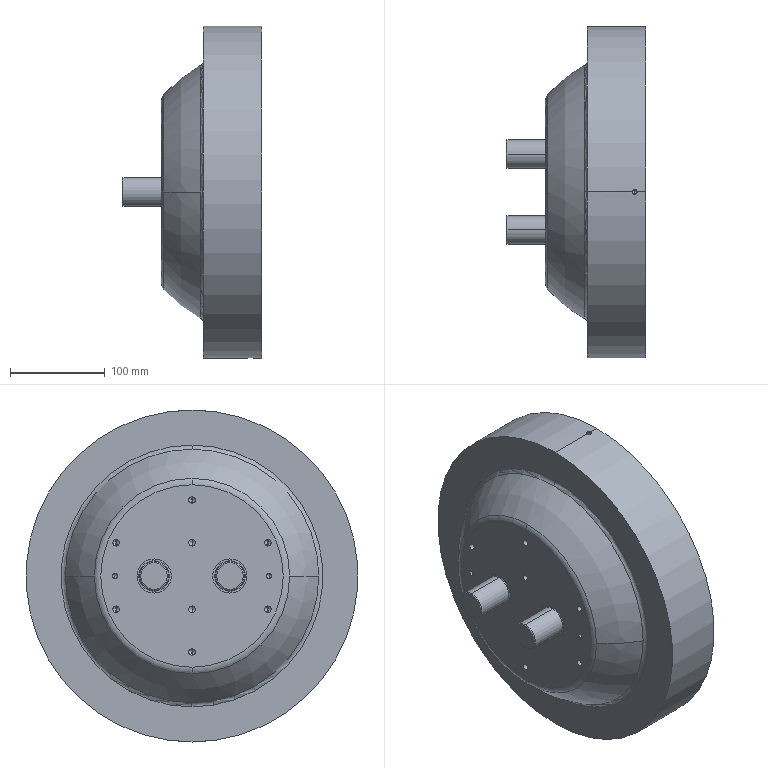Part | NX | features BREP 1 | 1 solid | 250 faces | box 147.5 x 350 x 350 mm | volume 7306362 mm3 | spline 79 | plane 69 | cylinder 48 | cone 40 | torus 12 | sphere 2 | commonest cylinder face diameters 6.8 x18 8.5 x8 4.5 x4 5 x4 30 x4 36 x4